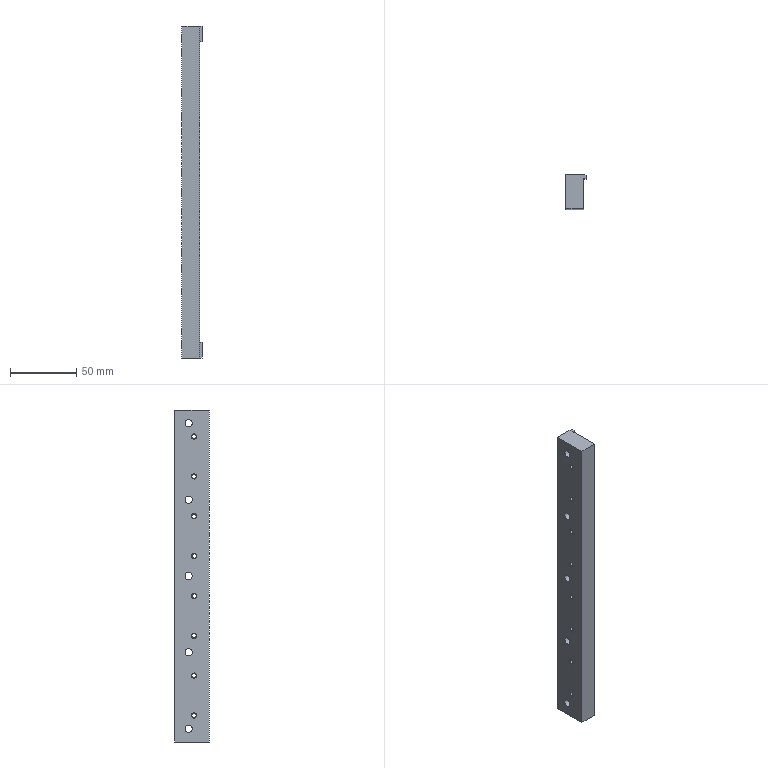Part | STEP file | 1 solid | 53 faces | box 15.5 x 26 x 250 mm | volume 83813 mm3 | plane 19 | cylinder 18 | cone 16 | commonest cylinder face diameters 3.242 x8 5.5 x5 10 x5